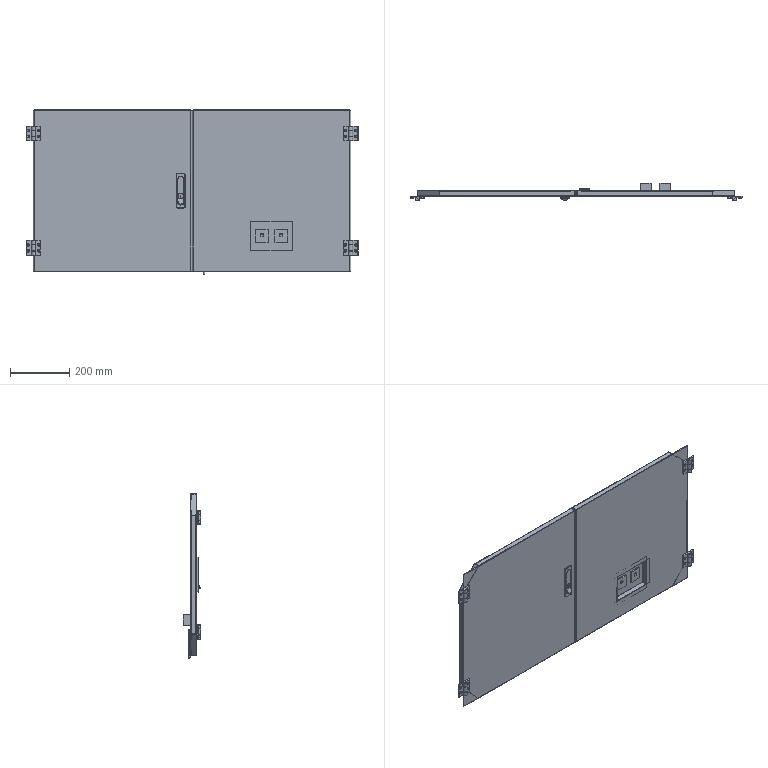Part | NX | features BREP 13 | 26 solids | 739 faces | box 1120 x 59.5 x 557.003 mm | volume 1312452 mm3 | plane 406 | cylinder 229 | sphere 40 | cone 34 | torus 22 | spline 8 | commonest cylinder face diameters 6 x54 4.4 x32 2 x27 3 x20 5 x16 10 x16